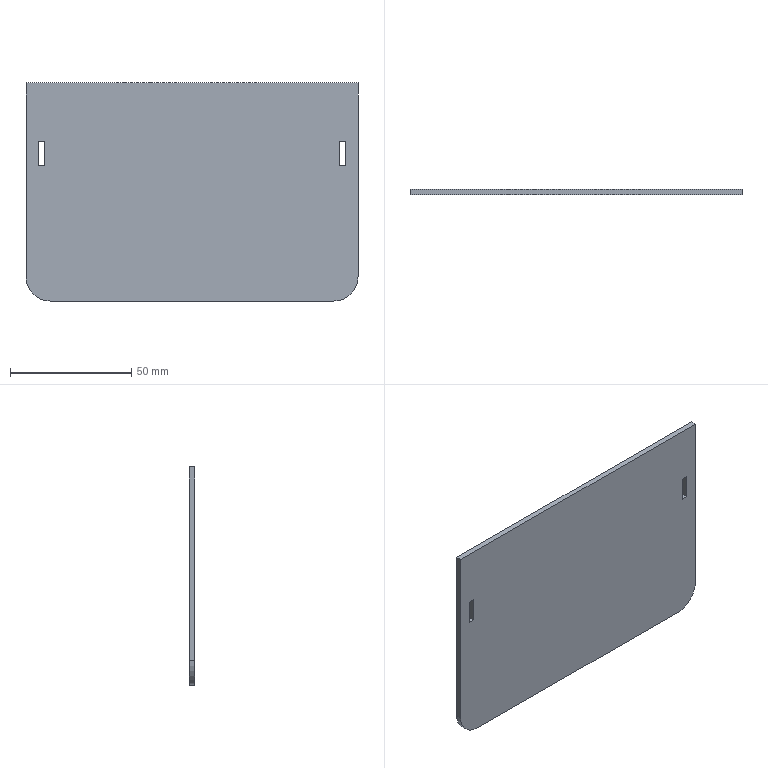Part | SolidWorks | features FlatPattern 1, SMBaseFlange 1, SheetMetal 1 | 1 solid | 16 faces | box 137 x 2.3 x 90 mm | volume 28143 mm3 | plane 14 | cylinder 2 | commonest cylinder face diameters 20 x2
STEP:
#1=CARTESIAN_POINT('',(68.5,0.,45.));
#2=VERTEX_POINT('',#1);
#3=CARTESIAN_POINT('',(68.5,0.,-35.));
#4=VERTEX_POINT('',#3);
#5=CARTESIAN_POINT('',(68.5,0.,-35.));
#6=DIRECTION('',(0.,0.,-1.));
#7=VECTOR('',#6,1000.);
#8=LINE('',#5,#7);
#9=EDGE_CURVE('',#2,#4,#8,.T.);
#10=ORIENTED_EDGE('',*,*,#9,.F.);
#11=CARTESIAN_POINT('',(68.5,-2.3,45.));
#12=VERTEX_POINT('',#11);
#13=CARTESIAN_POINT('',(68.5,-2.3,45.));
#14=DIRECTION('',(0.,1.,0.));
#15=VECTOR('',#14,1000.);
#16=LINE('',#13,#15);
#17=EDGE_CURVE('',#12,#2,#16,.T.);
#18=ORIENTED_EDGE('',*,*,#17,.F.);
#19=CARTESIAN_POINT('',(68.5,-2.3,-35.));
#20=VERTEX_POINT('',#19);
#21=CARTESIAN_POINT('',(68.5,-2.3,-35.));
#22=DIRECTION('',(0.,0.,-1.));
#23=VECTOR('',#22,1000.);
#24=LINE('',#21,#23);
#25=EDGE_CURVE('',#12,#20,#24,.T.);
#26=ORIENTED_EDGE('',*,*,#25,.T.);
#27=CARTESIAN_POINT('',(68.5,-2.3,-35.));
#28=DIRECTION('',(0.,1.,0.));
#29=VECTOR('',#28,1000.);
#30=LINE('',#27,#29);
#31=EDGE_CURVE('',#20,#4,#30,.T.);
#32=ORIENTED_EDGE('',*,*,#31,.T.);
#33=EDGE_LOOP('',(#10,#18,#26,#32));
#34=FACE_OUTER_BOUND('',#33,.T.);
#35=CARTESIAN_POINT('',(68.5,-2.3,-35.));
#36=DIRECTION('',(1.,0.,0.));
#37=DIRECTION('',(0.,0.,-1.));
#38=AXIS2_PLACEMENT_3D('',#35,#36,#37);
#39=PLANE('',#38);
#40=ADVANCED_FACE('',(#34),#39,.T.);
#41=CARTESIAN_POINT('',(-68.5,0.,45.));
#42=VERTEX_POINT('',#41);
#43=CARTESIAN_POINT('',(-68.5,0.,45.));
#44=DIRECTION('',(1.,0.,0.));
#45=VECTOR('',#44,1000.);
#46=LINE('',#43,#45);
#47=EDGE_CURVE('',#42,#2,#46,.T.);
#48=ORIENTED_EDGE('',*,*,#47,.F.);
#49=CARTESIAN_POINT('',(-68.5,-2.3,45.));
#50=VERTEX_POINT('',#49);
#51=CARTESIAN_POINT('',(-68.5,-2.3,45.));
#52=DIRECTION('',(0.,1.,0.));
#53=VECTOR('',#52,1000.);
#54=LINE('',#51,#53);
#55=EDGE_CURVE('',#50,#42,#54,.T.);
#56=ORIENTED_EDGE('',*,*,#55,.F.);
#57=CARTESIAN_POINT('',(-68.5,-2.3,45.));
#58=DIRECTION('',(1.,0.,0.));
#59=VECTOR('',#58,1000.);
#60=LINE('',#57,#59);
#61=EDGE_CURVE('',#50,#12,#60,.T.);
#62=ORIENTED_EDGE('',*,*,#61,.T.);
#63=ORIENTED_EDGE('',*,*,#17,.T.);
#64=EDGE_LOOP('',(#48,#56,#62,#63));
#65=FACE_OUTER_BOUND('',#64,.T.);
#66=CARTESIAN_POINT('',(-68.5,-2.3,45.));
#67=DIRECTION('',(0.,0.,1.));
#68=DIRECTION('',(1.,0.,0.));
#69=AXIS2_PLACEMENT_3D('',#66,#67,#68);
#70=PLANE('',#69);
#71=ADVANCED_FACE('',(#65),#70,.T.);
#72=CARTESIAN_POINT('',(-68.5,0.,-35.));
#73=VERTEX_POINT('',#72);
#74=CARTESIAN_POINT('',(-68.5,0.,-35.));
#75=DIRECTION('',(0.,0.,1.));
#76=VECTOR('',#75,1000.);
#77=LINE('',#74,#76);
#78=EDGE_CURVE('',#73,#42,#77,.T.);
#79=ORIENTED_EDGE('',*,*,#78,.F.);
#80=CARTESIAN_POINT('',(-68.5,-2.3,-35.));
#81=VERTEX_POINT('',#80);
#82=CARTESIAN_POINT('',(-68.5,-2.3,-35.));
#83=DIRECTION('',(0.,1.,0.));
#84=VECTOR('',#83,1000.);
#85=LINE('',#82,#84);
#86=EDGE_CURVE('',#81,#73,#85,.T.);
#87=ORIENTED_EDGE('',*,*,#86,.F.);
#88=CARTESIAN_POINT('',(-68.5,-2.3,-35.));
#89=DIRECTION('',(0.,0.,1.));
#90=VECTOR('',#89,1000.);
#91=LINE('',#88,#90);
#92=EDGE_CURVE('',#81,#50,#91,.T.);
#93=ORIENTED_EDGE('',*,*,#92,.T.);
#94=ORIENTED_EDGE('',*,*,#55,.T.);
#95=EDGE_LOOP('',(#79,#87,#93,#94));
#96=FACE_OUTER_BOUND('',#95,.T.);
#97=CARTESIAN_POINT('',(-68.5,-2.3,-35.));
#98=DIRECTION('',(-1.,0.,0.));
#99=DIRECTION('',(0.,0.,1.));
#100=AXIS2_PLACEMENT_3D('',#97,#98,#99);
#101=PLANE('',#100);
#102=ADVANCED_FACE('',(#96),#101,.T.);
#103=CARTESIAN_POINT('',(-58.5,0.,-45.));
#104=VERTEX_POINT('',#103);
#105=CARTESIAN_POINT('',(-58.5,0.,-35.));
#106=DIRECTION('',(0.,1.,0.));
#107=DIRECTION('',(0.,0.,1.));
#108=AXIS2_PLACEMENT_3D('',#105,#106,#107);
#109=CIRCLE('',#108,10.);
#110=EDGE_CURVE('',#104,#73,#109,.T.);
#111=ORIENTED_EDGE('',*,*,#110,.F.);
#112=CARTESIAN_POINT('',(-58.5,-2.3,-45.));
#113=VERTEX_POINT('',#112);
#114=CARTESIAN_POINT('',(-58.5,-2.3,-45.));
#115=DIRECTION('',(0.,1.,0.));
#116=VECTOR('',#115,1000.);
#117=LINE('',#114,#116);
#118=EDGE_CURVE('',#113,#104,#117,.T.);
#119=ORIENTED_EDGE('',*,*,#118,.F.);
#120=CARTESIAN_POINT('',(-58.5,-2.3,-35.));
#121=DIRECTION('',(0.,1.,0.));
#122=DIRECTION('',(0.,0.,1.));
#123=AXIS2_PLACEMENT_3D('',#120,#121,#122);
#124=CIRCLE('',#123,10.);
#125=EDGE_CURVE('',#113,#81,#124,.T.);
#126=ORIENTED_EDGE('',*,*,#125,.T.);
#127=ORIENTED_EDGE('',*,*,#86,.T.);
#128=EDGE_LOOP('',(#111,#119,#126,#127));
#129=FACE_OUTER_BOUND('',#128,.T.);
#130=CARTESIAN_POINT('',(-58.5,-2.3,-35.));
#131=DIRECTION('',(0.,1.,0.));
#132=DIRECTION('',(0.,0.,1.));
#133=AXIS2_PLACEMENT_3D('',#130,#131,#132);
#134=CYLINDRICAL_SURFACE('',#133,10.);
#135=ADVANCED_FACE('',(#129),#134,.T.);
#136=CARTESIAN_POINT('',(58.5,0.,-45.));
#137=VERTEX_POINT('',#136);
#138=CARTESIAN_POINT('',(-58.5,0.,-45.));
#139=DIRECTION('',(-1.,0.,0.));
#140=VECTOR('',#139,1000.);
#141=LINE('',#138,#140);
#142=EDGE_CURVE('',#137,#104,#141,.T.);
#143=ORIENTED_EDGE('',*,*,#142,.F.);
#144=CARTESIAN_POINT('',(58.5,-2.3,-45.));
#145=VERTEX_POINT('',#144);
#146=CARTESIAN_POINT('',(58.5,-2.3,-45.));
#147=DIRECTION('',(0.,1.,0.));
#148=VECTOR('',#147,1000.);
#149=LINE('',#146,#148);
#150=EDGE_CURVE('',#145,#137,#149,.T.);
#151=ORIENTED_EDGE('',*,*,#150,.F.);
#152=CARTESIAN_POINT('',(-58.5,-2.3,-45.));
#153=DIRECTION('',(-1.,0.,0.));
#154=VECTOR('',#153,1000.);
#155=LINE('',#152,#154);
#156=EDGE_CURVE('',#145,#113,#155,.T.);
#157=ORIENTED_EDGE('',*,*,#156,.T.);
#158=ORIENTED_EDGE('',*,*,#118,.T.);
#159=EDGE_LOOP('',(#143,#151,#157,#158));
#160=FACE_OUTER_BOUND('',#159,.T.);
#161=CARTESIAN_POINT('',(-58.5,-2.3,-45.));
#162=DIRECTION('',(0.,0.,-1.));
#163=DIRECTION('',(-1.,0.,0.));
#164=AXIS2_PLACEMENT_3D('',#161,#162,#163);
#165=PLANE('',#164);
#166=ADVANCED_FACE('',(#160),#165,.T.);
#167=CARTESIAN_POINT('',(58.5,0.,-35.));
#168=DIRECTION('',(0.,1.,0.));
#169=DIRECTION('',(0.,0.,-1.));
#170=AXIS2_PLACEMENT_3D('',#167,#168,#169);
#171=CIRCLE('',#170,10.);
#172=EDGE_CURVE('',#4,#137,#171,.T.);
#173=ORIENTED_EDGE('',*,*,#172,.F.);
#174=ORIENTED_EDGE('',*,*,#31,.F.);
#175=CARTESIAN_POINT('',(58.5,-2.3,-35.));
#176=DIRECTION('',(0.,1.,0.));
#177=DIRECTION('',(0.,0.,-1.));
#178=AXIS2_PLACEMENT_3D('',#175,#176,#177);
#179=CIRCLE('',#178,10.);
#180=EDGE_CURVE('',#20,#145,#179,.T.);
#181=ORIENTED_EDGE('',*,*,#180,.T.);
#182=ORIENTED_EDGE('',*,*,#150,.T.);
#183=EDGE_LOOP('',(#173,#174,#181,#182));
#184=FACE_OUTER_BOUND('',#183,.T.);
#185=CARTESIAN_POINT('',(58.5,-2.3,-35.));
#186=DIRECTION('',(0.,1.,0.));
#187=DIRECTION('',(0.,0.,1.));
#188=AXIS2_PLACEMENT_3D('',#185,#186,#187);
#189=CYLINDRICAL_SURFACE('',#188,10.);
#190=ADVANCED_FACE('',(#184),#189,.T.);
#191=CARTESIAN_POINT('',(63.5,-2.3,10.8));
#192=VERTEX_POINT('',#191);
#193=CARTESIAN_POINT('',(61.,-2.3,10.8));
#194=VERTEX_POINT('',#193);
#195=CARTESIAN_POINT('',(61.,-2.3,10.8));
#196=DIRECTION('',(-1.,0.,0.));
#197=VECTOR('',#196,1000.);
#198=LINE('',#195,#197);
#199=EDGE_CURVE('',#192,#194,#198,.T.);
#200=ORIENTED_EDGE('',*,*,#199,.T.);
#201=CARTESIAN_POINT('',(61.,-2.3,21.));
#202=VERTEX_POINT('',#201);
#203=CARTESIAN_POINT('',(61.,-2.3,10.8));
#204=DIRECTION('',(0.,0.,1.));
#205=VECTOR('',#204,1000.);
#206=LINE('',#203,#205);
#207=EDGE_CURVE('',#194,#202,#206,.T.);
#208=ORIENTED_EDGE('',*,*,#207,.T.);
#209=CARTESIAN_POINT('',(63.5,-2.3,21.));
#210=VERTEX_POINT('',#209);
#211=CARTESIAN_POINT('',(61.,-2.3,21.));
#212=DIRECTION('',(1.,0.,0.));
#213=VECTOR('',#212,1000.);
#214=LINE('',#211,#213);
#215=EDGE_CURVE('',#202,#210,#214,.T.);
#216=ORIENTED_EDGE('',*,*,#215,.T.);
#217=CARTESIAN_POINT('',(63.5,-2.3,10.8));
#218=DIRECTION('',(0.,0.,-1.));
#219=VECTOR('',#218,1000.);
#220=LINE('',#217,#219);
#221=EDGE_CURVE('',#210,#192,#220,.T.);
#222=ORIENTED_EDGE('',*,*,#221,.T.);
#223=EDGE_LOOP('',(#200,#208,#216,#222));
#224=FACE_BOUND('',#223,.T.);
#225=CARTESIAN_POINT('',(-61.,-2.3,10.8));
#226=VERTEX_POINT('',#225);
#227=CARTESIAN_POINT('',(-63.5,-2.3,10.8));
#228=VERTEX_POINT('',#227);
#229=CARTESIAN_POINT('',(-63.5,-2.3,10.8));
#230=DIRECTION('',(-1.,0.,0.));
#231=VECTOR('',#230,1000.);
#232=LINE('',#229,#231);
#233=EDGE_CURVE('',#226,#228,#232,.T.);
#234=ORIENTED_EDGE('',*,*,#233,.T.);
#235=CARTESIAN_POINT('',(-63.5,-2.3,21.));
#236=VERTEX_POINT('',#235);
#237=CARTESIAN_POINT('',(-63.5,-2.3,10.8));
#238=DIRECTION('',(0.,0.,1.));
#239=VECTOR('',#238,1000.);
#240=LINE('',#237,#239);
#241=EDGE_CURVE('',#228,#236,#240,.T.);
#242=ORIENTED_EDGE('',*,*,#241,.T.);
#243=CARTESIAN_POINT('',(-61.,-2.3,21.));
#244=VERTEX_POINT('',#243);
#245=CARTESIAN_POINT('',(-63.5,-2.3,21.));
#246=DIRECTION('',(1.,0.,0.));
#247=VECTOR('',#246,1000.);
#248=LINE('',#245,#247);
#249=EDGE_CURVE('',#236,#244,#248,.T.);
#250=ORIENTED_EDGE('',*,*,#249,.T.);
#251=CARTESIAN_POINT('',(-61.,-2.3,10.8));
#252=DIRECTION('',(0.,0.,-1.));
#253=VECTOR('',#252,1000.);
#254=LINE('',#251,#253);
#255=EDGE_CURVE('',#244,#226,#254,.T.);
#256=ORIENTED_EDGE('',*,*,#255,.T.);
#257=EDGE_LOOP('',(#234,#242,#250,#256));
#258=FACE_BOUND('',#257,.T.);
#259=ORIENTED_EDGE('',*,*,#25,.F.);
#260=ORIENTED_EDGE('',*,*,#61,.F.);
#261=ORIENTED_EDGE('',*,*,#92,.F.);
#262=ORIENTED_EDGE('',*,*,#125,.F.);
#263=ORIENTED_EDGE('',*,*,#156,.F.);
#264=ORIENTED_EDGE('',*,*,#180,.F.);
#265=EDGE_LOOP('',(#259,#260,#261,#262,#263,#264));
#266=FACE_OUTER_BOUND('',#265,.T.);
#267=CARTESIAN_POINT('',(-58.5,-2.3,-35.));
#268=DIRECTION('',(0.,1.,0.));
#269=DIRECTION('',(0.,0.,1.));
#270=AXIS2_PLACEMENT_3D('',#267,#268,#269);
#271=PLANE('',#270);
#272=ADVANCED_FACE('',(#224,#258,#266),#271,.F.);
#273=CARTESIAN_POINT('',(61.,0.,10.8));
#274=VERTEX_POINT('',#273);
#275=CARTESIAN_POINT('',(61.,0.,21.));
#276=VERTEX_POINT('',#275);
#277=CARTESIAN_POINT('',(61.,0.,10.8));
#278=DIRECTION('',(0.,0.,1.));
#279=VECTOR('',#278,1000.);
#280=LINE('',#277,#279);
#281=EDGE_CURVE('',#274,#276,#280,.T.);
#282=ORIENTED_EDGE('',*,*,#281,.F.);
#283=CARTESIAN_POINT('',(63.5,0.,10.8));
#284=VERTEX_POINT('',#283);
#285=CARTESIAN_POINT('',(61.,0.,10.8));
#286=DIRECTION('',(-1.,0.,0.));
#287=VECTOR('',#286,1000.);
#288=LINE('',#285,#287);
#289=EDGE_CURVE('',#284,#274,#288,.T.);
#290=ORIENTED_EDGE('',*,*,#289,.F.);
#291=CARTESIAN_POINT('',(63.5,0.,21.));
#292=VERTEX_POINT('',#291);
#293=CARTESIAN_POINT('',(63.5,0.,10.8));
#294=DIRECTION('',(0.,0.,-1.));
#295=VECTOR('',#294,1000.);
#296=LINE('',#293,#295);
#297=EDGE_CURVE('',#292,#284,#296,.T.);
#298=ORIENTED_EDGE('',*,*,#297,.F.);
#299=CARTESIAN_POINT('',(61.,0.,21.));
#300=DIRECTION('',(1.,0.,0.));
#301=VECTOR('',#300,1000.);
#302=LINE('',#299,#301);
#303=EDGE_CURVE('',#276,#292,#302,.T.);
#304=ORIENTED_EDGE('',*,*,#303,.F.);
#305=EDGE_LOOP('',(#282,#290,#298,#304));
#306=FACE_BOUND('',#305,.T.);
#307=CARTESIAN_POINT('',(-63.5,0.,10.8));
#308=VERTEX_POINT('',#307);
#309=CARTESIAN_POINT('',(-63.5,0.,21.));
#310=VERTEX_POINT('',#309);
#311=CARTESIAN_POINT('',(-63.5,0.,10.8));
#312=DIRECTION('',(0.,0.,1.));
#313=VECTOR('',#312,1000.);
#314=LINE('',#311,#313);
#315=EDGE_CURVE('',#308,#310,#314,.T.);
#316=ORIENTED_EDGE('',*,*,#315,.F.);
#317=CARTESIAN_POINT('',(-61.,0.,10.8));
#318=VERTEX_POINT('',#317);
#319=CARTESIAN_POINT('',(-63.5,0.,10.8));
#320=DIRECTION('',(-1.,0.,0.));
#321=VECTOR('',#320,1000.);
#322=LINE('',#319,#321);
#323=EDGE_CURVE('',#318,#308,#322,.T.);
#324=ORIENTED_EDGE('',*,*,#323,.F.);
#325=CARTESIAN_POINT('',(-61.,0.,21.));
#326=VERTEX_POINT('',#325);
#327=CARTESIAN_POINT('',(-61.,0.,10.8));
#328=DIRECTION('',(0.,0.,-1.));
#329=VECTOR('',#328,1000.);
#330=LINE('',#327,#329);
#331=EDGE_CURVE('',#326,#318,#330,.T.);
#332=ORIENTED_EDGE('',*,*,#331,.F.);
#333=CARTESIAN_POINT('',(-63.5,0.,21.));
#334=DIRECTION('',(1.,0.,0.));
#335=VECTOR('',#334,1000.);
#336=LINE('',#333,#335);
#337=EDGE_CURVE('',#310,#326,#336,.T.);
#338=ORIENTED_EDGE('',*,*,#337,.F.);
#339=EDGE_LOOP('',(#316,#324,#332,#338));
#340=FACE_BOUND('',#339,.T.);
#341=ORIENTED_EDGE('',*,*,#9,.T.);
#342=ORIENTED_EDGE('',*,*,#172,.T.);
#343=ORIENTED_EDGE('',*,*,#142,.T.);
#344=ORIENTED_EDGE('',*,*,#110,.T.);
#345=ORIENTED_EDGE('',*,*,#78,.T.);
#346=ORIENTED_EDGE('',*,*,#47,.T.);
#347=EDGE_LOOP('',(#341,#342,#343,#344,#345,#346));
#348=FACE_OUTER_BOUND('',#347,.T.);
#349=CARTESIAN_POINT('',(-58.5,0.,-35.));
#350=DIRECTION('',(0.,1.,0.));
#351=DIRECTION('',(0.,0.,1.));
#352=AXIS2_PLACEMENT_3D('',#349,#350,#351);
#353=PLANE('',#352);
#354=ADVANCED_FACE('',(#306,#340,#348),#353,.T.);
#355=ORIENTED_EDGE('',*,*,#315,.T.);
#356=CARTESIAN_POINT('',(-63.5,-2.3,21.));
#357=DIRECTION('',(0.,1.,0.));
#358=VECTOR('',#357,1000.);
#359=LINE('',#356,#358);
#360=EDGE_CURVE('',#236,#310,#359,.T.);
#361=ORIENTED_EDGE('',*,*,#360,.F.);
#362=ORIENTED_EDGE('',*,*,#241,.F.);
#363=CARTESIAN_POINT('',(-63.5,-2.3,10.8));
#364=DIRECTION('',(0.,1.,0.));
#365=VECTOR('',#364,1000.);
#366=LINE('',#363,#365);
#367=EDGE_CURVE('',#228,#308,#366,.T.);
#368=ORIENTED_EDGE('',*,*,#367,.T.);
#369=EDGE_LOOP('',(#355,#361,#362,#368));
#370=FACE_OUTER_BOUND('',#369,.T.);
#371=CARTESIAN_POINT('',(-63.5,-2.3,10.8));
#372=DIRECTION('',(-1.,0.,0.));
#373=DIRECTION('',(0.,0.,1.));
#374=AXIS2_PLACEMENT_3D('',#371,#372,#373);
#375=PLANE('',#374);
#376=ADVANCED_FACE('',(#370),#375,.F.);
#377=ORIENTED_EDGE('',*,*,#323,.T.);
#378=ORIENTED_EDGE('',*,*,#367,.F.);
#379=ORIENTED_EDGE('',*,*,#233,.F.);
#380=CARTESIAN_POINT('',(-61.,-2.3,10.8));
#381=DIRECTION('',(0.,1.,0.));
#382=VECTOR('',#381,1000.);
#383=LINE('',#380,#382);
#384=EDGE_CURVE('',#226,#318,#383,.T.);
#385=ORIENTED_EDGE('',*,*,#384,.T.);
#386=EDGE_LOOP('',(#377,#378,#379,#385));
#387=FACE_OUTER_BOUND('',#386,.T.);
#388=CARTESIAN_POINT('',(-63.5,-2.3,10.8));
#389=DIRECTION('',(0.,0.,-1.));
#390=DIRECTION('',(-1.,0.,0.));
#391=AXIS2_PLACEMENT_3D('',#388,#389,#390);
#392=PLANE('',#391);
#393=ADVANCED_FACE('',(#387),#392,.F.);
#394=ORIENTED_EDGE('',*,*,#331,.T.);
#395=ORIENTED_EDGE('',*,*,#384,.F.);
#396=ORIENTED_EDGE('',*,*,#255,.F.);
#397=CARTESIAN_POINT('',(-61.,-2.3,21.));
#398=DIRECTION('',(0.,1.,0.));
#399=VECTOR('',#398,1000.);
#400=LINE('',#397,#399);
#401=EDGE_CURVE('',#244,#326,#400,.T.);
#402=ORIENTED_EDGE('',*,*,#401,.T.);
#403=EDGE_LOOP('',(#394,#395,#396,#402));
#404=FACE_OUTER_BOUND('',#403,.T.);
#405=CARTESIAN_POINT('',(-61.,-2.3,10.8));
#406=DIRECTION('',(1.,0.,0.));
#407=DIRECTION('',(0.,0.,-1.));
#408=AXIS2_PLACEMENT_3D('',#405,#406,#407);
#409=PLANE('',#408);
#410=ADVANCED_FACE('',(#404),#409,.F.);
#411=ORIENTED_EDGE('',*,*,#337,.T.);
#412=ORIENTED_EDGE('',*,*,#401,.F.);
#413=ORIENTED_EDGE('',*,*,#249,.F.);
#414=ORIENTED_EDGE('',*,*,#360,.T.);
#415=EDGE_LOOP('',(#411,#412,#413,#414));
#416=FACE_OUTER_BOUND('',#415,.T.);
#417=CARTESIAN_POINT('',(-63.5,-2.3,21.));
#418=DIRECTION('',(0.,0.,1.));
#419=DIRECTION('',(1.,0.,0.));
#420=AXIS2_PLACEMENT_3D('',#417,#418,#419);
#421=PLANE('',#420);
#422=ADVANCED_FACE('',(#416),#421,.F.);
#423=ORIENTED_EDGE('',*,*,#281,.T.);
#424=CARTESIAN_POINT('',(61.,-2.3,21.));
#425=DIRECTION('',(0.,1.,0.));
#426=VECTOR('',#425,1000.);
#427=LINE('',#424,#426);
#428=EDGE_CURVE('',#202,#276,#427,.T.);
#429=ORIENTED_EDGE('',*,*,#428,.F.);
#430=ORIENTED_EDGE('',*,*,#207,.F.);
#431=CARTESIAN_POINT('',(61.,-2.3,10.8));
#432=DIRECTION('',(0.,1.,0.));
#433=VECTOR('',#432,1000.);
#434=LINE('',#431,#433);
#435=EDGE_CURVE('',#194,#274,#434,.T.);
#436=ORIENTED_EDGE('',*,*,#435,.T.);
#437=EDGE_LOOP('',(#423,#429,#430,#436));
#438=FACE_OUTER_BOUND('',#437,.T.);
#439=CARTESIAN_POINT('',(61.,-2.3,10.8));
#440=DIRECTION('',(-1.,0.,0.));
#441=DIRECTION('',(0.,0.,1.));
#442=AXIS2_PLACEMENT_3D('',#439,#440,#441);
#443=PLANE('',#442);
#444=ADVANCED_FACE('',(#438),#443,.F.);
#445=ORIENTED_EDGE('',*,*,#289,.T.);
#446=ORIENTED_EDGE('',*,*,#435,.F.);
#447=ORIENTED_EDGE('',*,*,#199,.F.);
#448=CARTESIAN_POINT('',(63.5,-2.3,10.8));
#449=DIRECTION('',(0.,1.,0.));
#450=VECTOR('',#449,1000.);
#451=LINE('',#448,#450);
#452=EDGE_CURVE('',#192,#284,#451,.T.);
#453=ORIENTED_EDGE('',*,*,#452,.T.);
#454=EDGE_LOOP('',(#445,#446,#447,#453));
#455=FACE_OUTER_BOUND('',#454,.T.);
#456=CARTESIAN_POINT('',(61.,-2.3,10.8));
#457=DIRECTION('',(0.,0.,-1.));
#458=DIRECTION('',(-1.,0.,0.));
#459=AXIS2_PLACEMENT_3D('',#456,#457,#458);
#460=PLANE('',#459);
#461=ADVANCED_FACE('',(#455),#460,.F.);
#462=ORIENTED_EDGE('',*,*,#297,.T.);
#463=ORIENTED_EDGE('',*,*,#452,.F.);
#464=ORIENTED_EDGE('',*,*,#221,.F.);
#465=CARTESIAN_POINT('',(63.5,-2.3,21.));
#466=DIRECTION('',(0.,1.,0.));
#467=VECTOR('',#466,1000.);
#468=LINE('',#465,#467);
#469=EDGE_CURVE('',#210,#292,#468,.T.);
#470=ORIENTED_EDGE('',*,*,#469,.T.);
#471=EDGE_LOOP('',(#462,#463,#464,#470));
#472=FACE_OUTER_BOUND('',#471,.T.);
#473=CARTESIAN_POINT('',(63.5,-2.3,10.8));
#474=DIRECTION('',(1.,0.,0.));
#475=DIRECTION('',(0.,0.,-1.));
#476=AXIS2_PLACEMENT_3D('',#473,#474,#475);
#477=PLANE('',#476);
#478=ADVANCED_FACE('',(#472),#477,.F.);
#479=ORIENTED_EDGE('',*,*,#303,.T.);
#480=ORIENTED_EDGE('',*,*,#469,.F.);
#481=ORIENTED_EDGE('',*,*,#215,.F.);
#482=ORIENTED_EDGE('',*,*,#428,.T.);
#483=EDGE_LOOP('',(#479,#480,#481,#482));
#484=FACE_OUTER_BOUND('',#483,.T.);
#485=CARTESIAN_POINT('',(61.,-2.3,21.));
#486=DIRECTION('',(0.,0.,1.));
#487=DIRECTION('',(1.,0.,0.));
#488=AXIS2_PLACEMENT_3D('',#485,#486,#487);
#489=PLANE('',#488);
#490=ADVANCED_FACE('',(#484),#489,.F.);
#491=CLOSED_SHELL('',(#40,#71,#102,#135,#166,#190,#272,#354,#376,#393,#410,#422,#444,#461,#478,#490));
#492=MANIFOLD_SOLID_BREP('',#491);
#493=CARTESIAN_POINT('',(0.,0.,0.));
#494=DIRECTION('',(0.,0.,1.));
#495=DIRECTION('',(1.,0.,0.));
#496=AXIS2_PLACEMENT_3D('',#493,#494,#495);
#497=(LENGTH_UNIT()NAMED_UNIT(*)SI_UNIT(.MILLI.,.METRE.));
#498=UNCERTAINTY_MEASURE_WITH_UNIT(LENGTH_MEASURE(0.00001),#497,'','');
#499=(NAMED_UNIT(*)PLANE_ANGLE_UNIT()SI_UNIT($,.RADIAN.));
#500=(NAMED_UNIT(*)SI_UNIT($,.STERADIAN.)SOLID_ANGLE_UNIT());
#501=(GEOMETRIC_REPRESENTATION_CONTEXT(3)GLOBAL_UNCERTAINTY_ASSIGNED_CONTEXT((#498))GLOBAL_UNIT_ASSIGNED_CONTEXT((#497,#499,#500))REPRESENTATION_CONTEXT('',''));
#502=ADVANCED_BREP_SHAPE_REPRESENTATION('',(#492,#496),#501);